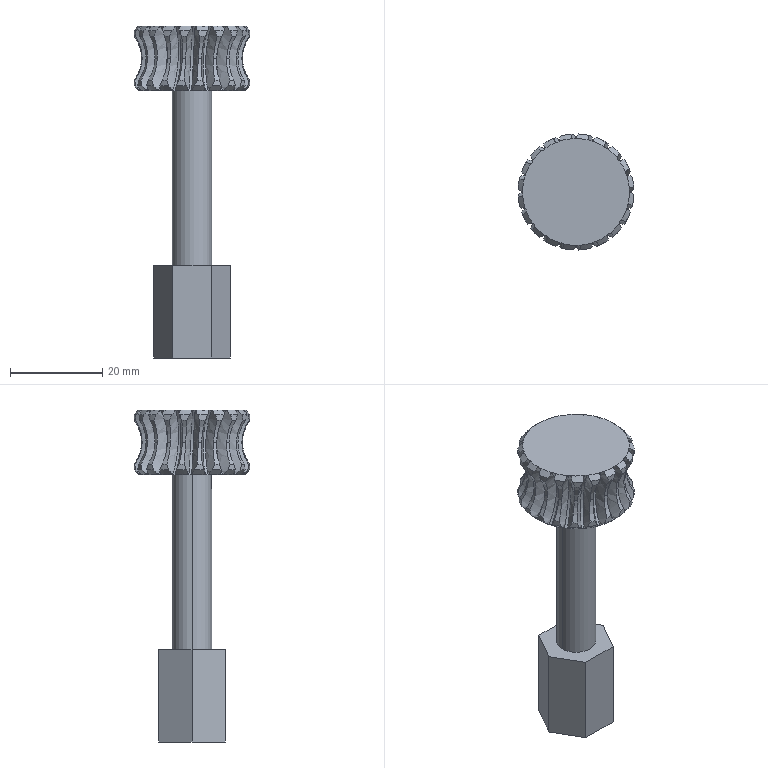Part | SolidWorks | features BaseBody 1 | 1 solid | 194 faces | box 25.14 x 25.14 x 72 mm | volume 10941 mm3 | spline 60 | cylinder 42 | cone 42 | torus 40 | plane 10 | commonest cylinder face diameters 25.162 x40 8.528 x2